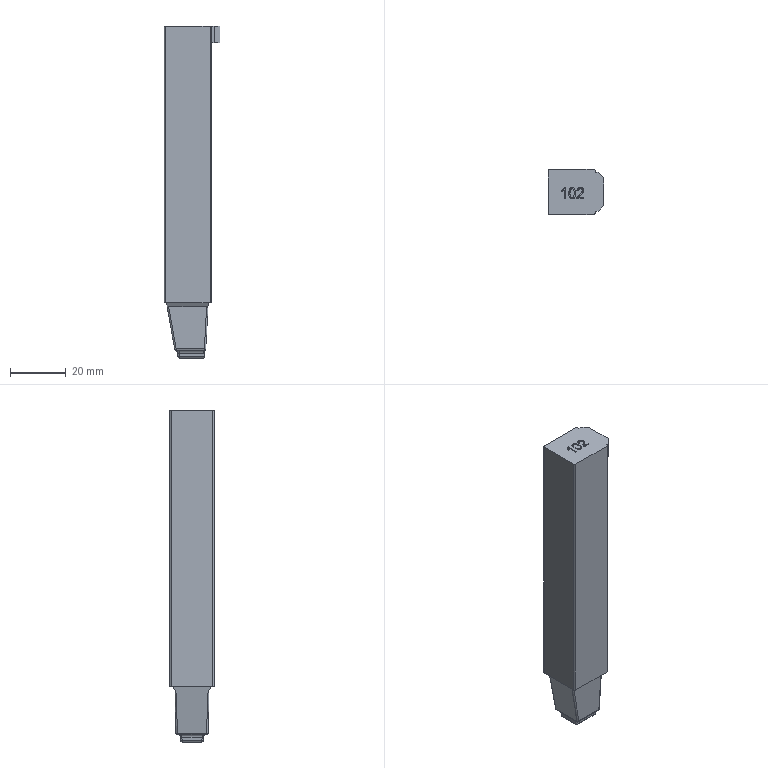Part | Creo | 1 solid | 100 faces | box 20 x 16 x 119.226 mm | volume 30103 mm3 | plane 44 | cylinder 24 | spline 16 | other 16 | commonest cylinder face diameters 1.002 x6 1.005 x5 1 x4 1.004 x4 2.211 x3 0.402 x2